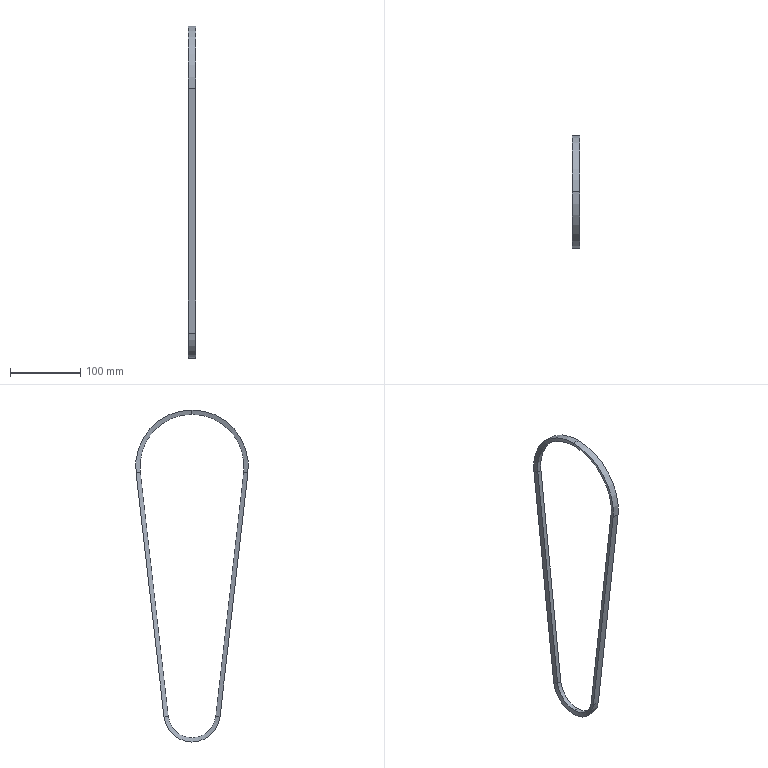Part | SolidWorks | features Sweep 1 | 1 solid | 22 faces | box 10 x 160 x 471.5 mm | volume 52282 mm3 | cylinder 8 | plane 8 | cone 6 | commonest cylinder face diameters 68 x2 80 x2 148 x2 160 x2
STEP:
#1=CARTESIAN_POINT('',(3.166,0.,74.));
#2=VERTEX_POINT('',#1);
#3=CARTESIAN_POINT('',(3.166,73.519,-8.421));
#4=VERTEX_POINT('',#3);
#5=CARTESIAN_POINT('',(3.166,0.,0.));
#6=DIRECTION('',(-1.,0.,0.));
#7=DIRECTION('',(0.,0.,1.));
#8=AXIS2_PLACEMENT_3D('',#5,#6,#7);
#9=CIRCLE('',#8,74.);
#10=EDGE_CURVE('',#2,#4,#9,.T.);
#11=ORIENTED_EDGE('',*,*,#10,.F.);
#12=CARTESIAN_POINT('',(-3.166,0.,74.));
#13=VERTEX_POINT('',#12);
#14=CARTESIAN_POINT('',(0.,0.,74.));
#15=DIRECTION('',(-1.,0.,0.));
#16=VECTOR('',#15,1000.);
#17=LINE('',#14,#16);
#18=EDGE_CURVE('',#2,#13,#17,.T.);
#19=ORIENTED_EDGE('',*,*,#18,.T.);
#20=CARTESIAN_POINT('',(-3.166,73.519,-8.421));
#21=VERTEX_POINT('',#20);
#22=CARTESIAN_POINT('',(-3.166,0.,0.));
#23=DIRECTION('',(-1.,0.,0.));
#24=DIRECTION('',(0.,0.,1.));
#25=AXIS2_PLACEMENT_3D('',#22,#23,#24);
#26=CIRCLE('',#25,74.);
#27=EDGE_CURVE('',#13,#21,#26,.T.);
#28=ORIENTED_EDGE('',*,*,#27,.T.);
#29=CARTESIAN_POINT('',(3.166,73.519,-8.421));
#30=DIRECTION('',(1.,0.,0.));
#31=VECTOR('',#30,1000.);
#32=LINE('',#29,#31);
#33=EDGE_CURVE('',#21,#4,#32,.T.);
#34=ORIENTED_EDGE('',*,*,#33,.T.);
#35=EDGE_LOOP('',(#11,#19,#28,#34));
#36=FACE_OUTER_BOUND('',#35,.T.);
#37=CARTESIAN_POINT('',(0.,0.,0.));
#38=DIRECTION('',(-1.,0.,0.));
#39=DIRECTION('',(0.,0.,1.));
#40=AXIS2_PLACEMENT_3D('',#37,#38,#39);
#41=CYLINDRICAL_SURFACE('',#40,74.);
#42=ADVANCED_FACE('',(#36),#41,.F.);
#43=CARTESIAN_POINT('',(5.,-79.48,-9.104));
#44=VERTEX_POINT('',#43);
#45=CARTESIAN_POINT('',(5.,0.,80.));
#46=VERTEX_POINT('',#45);
#47=CARTESIAN_POINT('',(5.,0.,0.));
#48=DIRECTION('',(-1.,0.,0.));
#49=DIRECTION('',(0.,0.,1.));
#50=AXIS2_PLACEMENT_3D('',#47,#48,#49);
#51=CIRCLE('',#50,80.);
#52=EDGE_CURVE('',#44,#46,#51,.T.);
#53=ORIENTED_EDGE('',*,*,#52,.T.);
#54=CARTESIAN_POINT('',(-5.,0.,80.));
#55=VERTEX_POINT('',#54);
#56=CARTESIAN_POINT('',(0.,0.,80.));
#57=DIRECTION('',(-1.,0.,0.));
#58=VECTOR('',#57,1000.);
#59=LINE('',#56,#58);
#60=EDGE_CURVE('',#46,#55,#59,.T.);
#61=ORIENTED_EDGE('',*,*,#60,.T.);
#62=CARTESIAN_POINT('',(-5.,-79.48,-9.104));
#63=VERTEX_POINT('',#62);
#64=CARTESIAN_POINT('',(-5.,0.,0.));
#65=DIRECTION('',(-1.,0.,0.));
#66=DIRECTION('',(0.,0.,1.));
#67=AXIS2_PLACEMENT_3D('',#64,#65,#66);
#68=CIRCLE('',#67,80.);
#69=EDGE_CURVE('',#63,#55,#68,.T.);
#70=ORIENTED_EDGE('',*,*,#69,.F.);
#71=CARTESIAN_POINT('',(-5.,-79.48,-9.104));
#72=DIRECTION('',(-1.,0.,0.));
#73=VECTOR('',#72,1000.);
#74=LINE('',#71,#73);
#75=EDGE_CURVE('',#44,#63,#74,.T.);
#76=ORIENTED_EDGE('',*,*,#75,.F.);
#77=EDGE_LOOP('',(#53,#61,#70,#76));
#78=FACE_OUTER_BOUND('',#77,.T.);
#79=CARTESIAN_POINT('',(0.,0.,0.));
#80=DIRECTION('',(-1.,0.,0.));
#81=DIRECTION('',(0.,0.,1.));
#82=AXIS2_PLACEMENT_3D('',#79,#80,#81);
#83=CYLINDRICAL_SURFACE('',#82,80.);
#84=ADVANCED_FACE('',(#78),#83,.T.);
#85=ORIENTED_EDGE('',*,*,#27,.F.);
#86=CARTESIAN_POINT('',(-5.,0.,80.));
#87=DIRECTION('',(-0.2924,0.,0.9563));
#88=VECTOR('',#87,1000.);
#89=LINE('',#86,#88);
#90=EDGE_CURVE('',#13,#55,#89,.T.);
#91=ORIENTED_EDGE('',*,*,#90,.T.);
#92=CARTESIAN_POINT('',(-5.,79.48,-9.104));
#93=VERTEX_POINT('',#92);
#94=CARTESIAN_POINT('',(-5.,0.,0.));
#95=DIRECTION('',(-1.,0.,0.));
#96=DIRECTION('',(0.,0.,1.));
#97=AXIS2_PLACEMENT_3D('',#94,#95,#96);
#98=CIRCLE('',#97,80.);
#99=EDGE_CURVE('',#55,#93,#98,.T.);
#100=ORIENTED_EDGE('',*,*,#99,.T.);
#101=CARTESIAN_POINT('',(-3.166,73.519,-8.421));
#102=DIRECTION('',(0.2924,-0.9501,0.1088));
#103=VECTOR('',#102,1000.);
#104=LINE('',#101,#103);
#105=EDGE_CURVE('',#93,#21,#104,.T.);
#106=ORIENTED_EDGE('',*,*,#105,.T.);
#107=EDGE_LOOP('',(#85,#91,#100,#106));
#108=FACE_OUTER_BOUND('',#107,.T.);
#109=CARTESIAN_POINT('',(-5.,0.,0.));
#110=DIRECTION('',(-1.,0.,0.));
#111=DIRECTION('',(0.,0.,1.));
#112=AXIS2_PLACEMENT_3D('',#109,#110,#111);
#113=CONICAL_SURFACE('',#112,80.,1.274);
#114=ADVANCED_FACE('',(#108),#113,.F.);
#115=CARTESIAN_POINT('',(-5.,-39.74,-356.052));
#116=VERTEX_POINT('',#115);
#117=CARTESIAN_POINT('',(-5.,0.,-391.5));
#118=VERTEX_POINT('',#117);
#119=CARTESIAN_POINT('',(-5.,0.,-351.5));
#120=DIRECTION('',(1.,0.,0.));
#121=DIRECTION('',(0.,0.,-1.));
#122=AXIS2_PLACEMENT_3D('',#119,#120,#121);
#123=CIRCLE('',#122,40.);
#124=EDGE_CURVE('',#116,#118,#123,.T.);
#125=ORIENTED_EDGE('',*,*,#124,.T.);
#126=CARTESIAN_POINT('',(5.,0.,-391.5));
#127=VERTEX_POINT('',#126);
#128=CARTESIAN_POINT('',(0.,0.,-391.5));
#129=DIRECTION('',(1.,0.,0.));
#130=VECTOR('',#129,1000.);
#131=LINE('',#128,#130);
#132=EDGE_CURVE('',#118,#127,#131,.T.);
#133=ORIENTED_EDGE('',*,*,#132,.T.);
#134=CARTESIAN_POINT('',(5.,-39.74,-356.052));
#135=VERTEX_POINT('',#134);
#136=CARTESIAN_POINT('',(5.,0.,-351.5));
#137=DIRECTION('',(1.,0.,0.));
#138=DIRECTION('',(0.,0.,-1.));
#139=AXIS2_PLACEMENT_3D('',#136,#137,#138);
#140=CIRCLE('',#139,40.);
#141=EDGE_CURVE('',#135,#127,#140,.T.);
#142=ORIENTED_EDGE('',*,*,#141,.F.);
#143=CARTESIAN_POINT('',(-5.,-39.74,-356.052));
#144=DIRECTION('',(-1.,0.,0.));
#145=VECTOR('',#144,1000.);
#146=LINE('',#143,#145);
#147=EDGE_CURVE('',#135,#116,#146,.T.);
#148=ORIENTED_EDGE('',*,*,#147,.T.);
#149=EDGE_LOOP('',(#125,#133,#142,#148));
#150=FACE_OUTER_BOUND('',#149,.T.);
#151=CARTESIAN_POINT('',(0.,0.,-351.5));
#152=DIRECTION('',(1.,0.,0.));
#153=DIRECTION('',(0.,0.,-1.));
#154=AXIS2_PLACEMENT_3D('',#151,#152,#153);
#155=CYLINDRICAL_SURFACE('',#154,40.);
#156=ADVANCED_FACE('',(#150),#155,.T.);
#157=CARTESIAN_POINT('',(3.166,0.,-385.5));
#158=VERTEX_POINT('',#157);
#159=CARTESIAN_POINT('',(3.166,33.779,-355.369));
#160=VERTEX_POINT('',#159);
#161=CARTESIAN_POINT('',(3.166,0.,-351.5));
#162=DIRECTION('',(1.,0.,0.));
#163=DIRECTION('',(0.,0.,-1.));
#164=AXIS2_PLACEMENT_3D('',#161,#162,#163);
#165=CIRCLE('',#164,34.);
#166=EDGE_CURVE('',#158,#160,#165,.T.);
#167=ORIENTED_EDGE('',*,*,#166,.F.);
#168=CARTESIAN_POINT('',(3.166,0.,-385.5));
#169=DIRECTION('',(0.2924,0.,-0.9563));
#170=VECTOR('',#169,1000.);
#171=LINE('',#168,#170);
#172=EDGE_CURVE('',#158,#127,#171,.T.);
#173=ORIENTED_EDGE('',*,*,#172,.T.);
#174=CARTESIAN_POINT('',(5.,39.74,-356.052));
#175=VERTEX_POINT('',#174);
#176=CARTESIAN_POINT('',(5.,0.,-351.5));
#177=DIRECTION('',(1.,0.,0.));
#178=DIRECTION('',(0.,0.,-1.));
#179=AXIS2_PLACEMENT_3D('',#176,#177,#178);
#180=CIRCLE('',#179,40.);
#181=EDGE_CURVE('',#127,#175,#180,.T.);
#182=ORIENTED_EDGE('',*,*,#181,.T.);
#183=CARTESIAN_POINT('',(5.,39.74,-356.052));
#184=DIRECTION('',(0.2924,0.9501,-0.1088));
#185=VECTOR('',#184,1000.);
#186=LINE('',#183,#185);
#187=EDGE_CURVE('',#160,#175,#186,.T.);
#188=ORIENTED_EDGE('',*,*,#187,.F.);
#189=EDGE_LOOP('',(#167,#173,#182,#188));
#190=FACE_OUTER_BOUND('',#189,.T.);
#191=CARTESIAN_POINT('',(3.166,0.,-351.5));
#192=DIRECTION('',(1.,0.,0.));
#193=DIRECTION('',(0.,0.,-1.));
#194=AXIS2_PLACEMENT_3D('',#191,#192,#193);
#195=CONICAL_SURFACE('',#194,34.,1.274);
#196=ADVANCED_FACE('',(#190),#195,.F.);
#197=CARTESIAN_POINT('',(-3.166,0.,-385.5));
#198=VERTEX_POINT('',#197);
#199=CARTESIAN_POINT('',(-3.166,33.779,-355.369));
#200=VERTEX_POINT('',#199);
#201=CARTESIAN_POINT('',(-3.166,0.,-351.5));
#202=DIRECTION('',(1.,0.,0.));
#203=DIRECTION('',(0.,0.,-1.));
#204=AXIS2_PLACEMENT_3D('',#201,#202,#203);
#205=CIRCLE('',#204,34.);
#206=EDGE_CURVE('',#198,#200,#205,.T.);
#207=ORIENTED_EDGE('',*,*,#206,.F.);
#208=CARTESIAN_POINT('',(0.,0.,-385.5));
#209=DIRECTION('',(1.,0.,0.));
#210=VECTOR('',#209,1000.);
#211=LINE('',#208,#210);
#212=EDGE_CURVE('',#198,#158,#211,.T.);
#213=ORIENTED_EDGE('',*,*,#212,.T.);
#214=ORIENTED_EDGE('',*,*,#166,.T.);
#215=CARTESIAN_POINT('',(3.166,33.779,-355.369));
#216=DIRECTION('',(1.,0.,0.));
#217=VECTOR('',#216,1000.);
#218=LINE('',#215,#217);
#219=EDGE_CURVE('',#200,#160,#218,.T.);
#220=ORIENTED_EDGE('',*,*,#219,.F.);
#221=EDGE_LOOP('',(#207,#213,#214,#220));
#222=FACE_OUTER_BOUND('',#221,.T.);
#223=CARTESIAN_POINT('',(0.,0.,-351.5));
#224=DIRECTION('',(1.,0.,0.));
#225=DIRECTION('',(0.,0.,-1.));
#226=AXIS2_PLACEMENT_3D('',#223,#224,#225);
#227=CYLINDRICAL_SURFACE('',#226,34.);
#228=ADVANCED_FACE('',(#222),#227,.F.);
#229=ORIENTED_EDGE('',*,*,#219,.T.);
#230=CARTESIAN_POINT('',(3.166,33.779,-355.369));
#231=DIRECTION('',(0.,0.1138,0.9935));
#232=VECTOR('',#231,1000.);
#233=LINE('',#230,#232);
#234=EDGE_CURVE('',#160,#4,#233,.T.);
#235=ORIENTED_EDGE('',*,*,#234,.T.);
#236=ORIENTED_EDGE('',*,*,#33,.F.);
#237=CARTESIAN_POINT('',(-3.166,33.779,-355.369));
#238=DIRECTION('',(0.,0.1138,0.9935));
#239=VECTOR('',#238,1000.);
#240=LINE('',#237,#239);
#241=EDGE_CURVE('',#200,#21,#240,.T.);
#242=ORIENTED_EDGE('',*,*,#241,.F.);
#243=EDGE_LOOP('',(#229,#235,#236,#242));
#244=FACE_OUTER_BOUND('',#243,.T.);
#245=CARTESIAN_POINT('',(3.166,33.779,-355.369));
#246=DIRECTION('',(0.,-0.9935,0.1138));
#247=DIRECTION('',(0.,-0.1138,-0.9935));
#248=AXIS2_PLACEMENT_3D('',#245,#246,#247);
#249=PLANE('',#248);
#250=ADVANCED_FACE('',(#244),#249,.T.);
#251=ORIENTED_EDGE('',*,*,#187,.T.);
#252=CARTESIAN_POINT('',(5.,79.48,-9.104));
#253=VERTEX_POINT('',#252);
#254=CARTESIAN_POINT('',(5.,39.74,-356.052));
#255=DIRECTION('',(0.,0.1138,0.9935));
#256=VECTOR('',#255,1000.);
#257=LINE('',#254,#256);
#258=EDGE_CURVE('',#175,#253,#257,.T.);
#259=ORIENTED_EDGE('',*,*,#258,.T.);
#260=CARTESIAN_POINT('',(5.,79.48,-9.104));
#261=DIRECTION('',(0.2924,0.9501,-0.1088));
#262=VECTOR('',#261,1000.);
#263=LINE('',#260,#262);
#264=EDGE_CURVE('',#4,#253,#263,.T.);
#265=ORIENTED_EDGE('',*,*,#264,.F.);
#266=ORIENTED_EDGE('',*,*,#234,.F.);
#267=EDGE_LOOP('',(#251,#259,#265,#266));
#268=FACE_OUTER_BOUND('',#267,.T.);
#269=CARTESIAN_POINT('',(5.,39.74,-356.052));
#270=DIRECTION('',(0.9563,-0.2905,0.03327));
#271=DIRECTION('',(0.2906,0.9568,0.));
#272=AXIS2_PLACEMENT_3D('',#269,#270,#271);
#273=PLANE('',#272);
#274=ADVANCED_FACE('',(#268),#273,.T.);
#275=CARTESIAN_POINT('',(-5.,39.74,-356.052));
#276=VERTEX_POINT('',#275);
#277=CARTESIAN_POINT('',(-5.,39.74,-356.052));
#278=DIRECTION('',(-1.,0.,0.));
#279=VECTOR('',#278,1000.);
#280=LINE('',#277,#279);
#281=EDGE_CURVE('',#175,#276,#280,.T.);
#282=ORIENTED_EDGE('',*,*,#281,.T.);
#283=CARTESIAN_POINT('',(-5.,39.74,-356.052));
#284=DIRECTION('',(0.,0.1138,0.9935));
#285=VECTOR('',#284,1000.);
#286=LINE('',#283,#285);
#287=EDGE_CURVE('',#276,#93,#286,.T.);
#288=ORIENTED_EDGE('',*,*,#287,.T.);
#289=CARTESIAN_POINT('',(-5.,79.48,-9.104));
#290=DIRECTION('',(-1.,0.,0.));
#291=VECTOR('',#290,1000.);
#292=LINE('',#289,#291);
#293=EDGE_CURVE('',#253,#93,#292,.T.);
#294=ORIENTED_EDGE('',*,*,#293,.F.);
#295=ORIENTED_EDGE('',*,*,#258,.F.);
#296=EDGE_LOOP('',(#282,#288,#294,#295));
#297=FACE_OUTER_BOUND('',#296,.T.);
#298=CARTESIAN_POINT('',(-5.,39.74,-356.052));
#299=DIRECTION('',(0.,0.9935,-0.1138));
#300=DIRECTION('',(0.,0.1138,0.9935));
#301=AXIS2_PLACEMENT_3D('',#298,#299,#300);
#302=PLANE('',#301);
#303=ADVANCED_FACE('',(#297),#302,.T.);
#304=CARTESIAN_POINT('',(-3.166,33.779,-355.369));
#305=DIRECTION('',(0.2924,-0.9501,0.1088));
#306=VECTOR('',#305,1000.);
#307=LINE('',#304,#306);
#308=EDGE_CURVE('',#276,#200,#307,.T.);
#309=ORIENTED_EDGE('',*,*,#308,.T.);
#310=ORIENTED_EDGE('',*,*,#241,.T.);
#311=ORIENTED_EDGE('',*,*,#105,.F.);
#312=ORIENTED_EDGE('',*,*,#287,.F.);
#313=EDGE_LOOP('',(#309,#310,#311,#312));
#314=FACE_OUTER_BOUND('',#313,.T.);
#315=CARTESIAN_POINT('',(-3.166,33.779,-355.369));
#316=DIRECTION('',(-0.9563,-0.2905,0.03327));
#317=DIRECTION('',(0.2906,-0.9568,0.));
#318=AXIS2_PLACEMENT_3D('',#315,#316,#317);
#319=PLANE('',#318);
#320=ADVANCED_FACE('',(#314),#319,.T.);
#321=ORIENTED_EDGE('',*,*,#212,.F.);
#322=CARTESIAN_POINT('',(-3.166,-33.779,-355.369));
#323=VERTEX_POINT('',#322);
#324=CARTESIAN_POINT('',(-3.166,0.,-351.5));
#325=DIRECTION('',(1.,0.,0.));
#326=DIRECTION('',(0.,0.,-1.));
#327=AXIS2_PLACEMENT_3D('',#324,#325,#326);
#328=CIRCLE('',#327,34.);
#329=EDGE_CURVE('',#323,#198,#328,.T.);
#330=ORIENTED_EDGE('',*,*,#329,.F.);
#331=CARTESIAN_POINT('',(3.166,-33.779,-355.369));
#332=VERTEX_POINT('',#331);
#333=CARTESIAN_POINT('',(3.166,-33.779,-355.369));
#334=DIRECTION('',(1.,0.,0.));
#335=VECTOR('',#334,1000.);
#336=LINE('',#333,#335);
#337=EDGE_CURVE('',#323,#332,#336,.T.);
#338=ORIENTED_EDGE('',*,*,#337,.T.);
#339=CARTESIAN_POINT('',(3.166,0.,-351.5));
#340=DIRECTION('',(1.,0.,0.));
#341=DIRECTION('',(0.,0.,-1.));
#342=AXIS2_PLACEMENT_3D('',#339,#340,#341);
#343=CIRCLE('',#342,34.);
#344=EDGE_CURVE('',#332,#158,#343,.T.);
#345=ORIENTED_EDGE('',*,*,#344,.T.);
#346=EDGE_LOOP('',(#321,#330,#338,#345));
#347=FACE_OUTER_BOUND('',#346,.T.);
#348=CARTESIAN_POINT('',(0.,0.,-351.5));
#349=DIRECTION('',(1.,0.,0.));
#350=DIRECTION('',(0.,0.,-1.));
#351=AXIS2_PLACEMENT_3D('',#348,#349,#350);
#352=CYLINDRICAL_SURFACE('',#351,34.);
#353=ADVANCED_FACE('',(#347),#352,.F.);
#354=ORIENTED_EDGE('',*,*,#172,.F.);
#355=ORIENTED_EDGE('',*,*,#344,.F.);
#356=CARTESIAN_POINT('',(5.,-39.74,-356.052));
#357=DIRECTION('',(0.2924,-0.9501,-0.1088));
#358=VECTOR('',#357,1000.);
#359=LINE('',#356,#358);
#360=EDGE_CURVE('',#332,#135,#359,.T.);
#361=ORIENTED_EDGE('',*,*,#360,.T.);
#362=ORIENTED_EDGE('',*,*,#141,.T.);
#363=EDGE_LOOP('',(#354,#355,#361,#362));
#364=FACE_OUTER_BOUND('',#363,.T.);
#365=CARTESIAN_POINT('',(3.166,0.,-351.5));
#366=DIRECTION('',(1.,0.,0.));
#367=DIRECTION('',(0.,0.,-1.));
#368=AXIS2_PLACEMENT_3D('',#365,#366,#367);
#369=CONICAL_SURFACE('',#368,34.,1.274);
#370=ADVANCED_FACE('',(#364),#369,.F.);
#371=ORIENTED_EDGE('',*,*,#132,.F.);
#372=CARTESIAN_POINT('',(-5.,0.,-351.5));
#373=DIRECTION('',(1.,0.,0.));
#374=DIRECTION('',(0.,0.,-1.));
#375=AXIS2_PLACEMENT_3D('',#372,#373,#374);
#376=CIRCLE('',#375,40.);
#377=EDGE_CURVE('',#118,#276,#376,.T.);
#378=ORIENTED_EDGE('',*,*,#377,.T.);
#379=ORIENTED_EDGE('',*,*,#281,.F.);
#380=ORIENTED_EDGE('',*,*,#181,.F.);
#381=EDGE_LOOP('',(#371,#378,#379,#380));
#382=FACE_OUTER_BOUND('',#381,.T.);
#383=CARTESIAN_POINT('',(0.,0.,-351.5));
#384=DIRECTION('',(1.,0.,0.));
#385=DIRECTION('',(0.,0.,-1.));
#386=AXIS2_PLACEMENT_3D('',#383,#384,#385);
#387=CYLINDRICAL_SURFACE('',#386,40.);
#388=ADVANCED_FACE('',(#382),#387,.T.);
#389=CARTESIAN_POINT('',(-3.166,-33.779,-355.369));
#390=DIRECTION('',(0.2924,0.9501,0.1088));
#391=VECTOR('',#390,1000.);
#392=LINE('',#389,#391);
#393=EDGE_CURVE('',#116,#323,#392,.T.);
#394=ORIENTED_EDGE('',*,*,#393,.T.);
#395=ORIENTED_EDGE('',*,*,#329,.T.);
#396=ORIENTED_EDGE('',*,*,#206,.T.);
#397=ORIENTED_EDGE('',*,*,#308,.F.);
#398=ORIENTED_EDGE('',*,*,#377,.F.);
#399=ORIENTED_EDGE('',*,*,#124,.F.);
#400=EDGE_LOOP('',(#394,#395,#396,#397,#398,#399));
#401=FACE_OUTER_BOUND('',#400,.T.);
#402=CARTESIAN_POINT('',(-5.,0.,-351.5));
#403=DIRECTION('',(-1.,0.,0.));
#404=DIRECTION('',(0.,0.,1.));
#405=AXIS2_PLACEMENT_3D('',#402,#403,#404);
#406=CONICAL_SURFACE('',#405,40.,1.274);
#407=ADVANCED_FACE('',(#401),#406,.F.);
#408=CARTESIAN_POINT('',(-3.166,-73.519,-8.421));
#409=VERTEX_POINT('',#408);
#410=CARTESIAN_POINT('',(3.166,-73.519,-8.421));
#411=VERTEX_POINT('',#410);
#412=CARTESIAN_POINT('',(3.166,-73.519,-8.421));
#413=DIRECTION('',(1.,0.,0.));
#414=VECTOR('',#413,1000.);
#415=LINE('',#412,#414);
#416=EDGE_CURVE('',#409,#411,#415,.T.);
#417=ORIENTED_EDGE('',*,*,#416,.T.);
#418=CARTESIAN_POINT('',(3.166,-73.519,-8.421));
#419=DIRECTION('',(0.,0.1138,-0.9935));
#420=VECTOR('',#419,1000.);
#421=LINE('',#418,#420);
#422=EDGE_CURVE('',#411,#332,#421,.T.);
#423=ORIENTED_EDGE('',*,*,#422,.T.);
#424=ORIENTED_EDGE('',*,*,#337,.F.);
#425=CARTESIAN_POINT('',(-3.166,-73.519,-8.421));
#426=DIRECTION('',(0.,0.1138,-0.9935));
#427=VECTOR('',#426,1000.);
#428=LINE('',#425,#427);
#429=EDGE_CURVE('',#409,#323,#428,.T.);
#430=ORIENTED_EDGE('',*,*,#429,.F.);
#431=EDGE_LOOP('',(#417,#423,#424,#430));
#432=FACE_OUTER_BOUND('',#431,.T.);
#433=CARTESIAN_POINT('',(3.166,-73.519,-8.421));
#434=DIRECTION('',(0.,0.9935,0.1138));
#435=DIRECTION('',(0.,-0.1138,0.9935));
#436=AXIS2_PLACEMENT_3D('',#433,#434,#435);
#437=PLANE('',#436);
#438=ADVANCED_FACE('',(#432),#437,.T.);
#439=CARTESIAN_POINT('',(5.,-79.48,-9.104));
#440=DIRECTION('',(0.2924,-0.9501,-0.1088));
#441=VECTOR('',#440,1000.);
#442=LINE('',#439,#441);
#443=EDGE_CURVE('',#411,#44,#442,.T.);
#444=ORIENTED_EDGE('',*,*,#443,.T.);
#445=CARTESIAN_POINT('',(5.,-79.48,-9.104));
#446=DIRECTION('',(0.,0.1138,-0.9935));
#447=VECTOR('',#446,1000.);
#448=LINE('',#445,#447);
#449=EDGE_CURVE('',#44,#135,#448,.T.);
#450=ORIENTED_EDGE('',*,*,#449,.T.);
#451=ORIENTED_EDGE('',*,*,#360,.F.);
#452=ORIENTED_EDGE('',*,*,#422,.F.);
#453=EDGE_LOOP('',(#444,#450,#451,#452));
#454=FACE_OUTER_BOUND('',#453,.T.);
#455=CARTESIAN_POINT('',(5.,-79.48,-9.104));
#456=DIRECTION('',(0.9563,0.2905,0.03327));
#457=DIRECTION('',(-0.2906,0.9568,0.));
#458=AXIS2_PLACEMENT_3D('',#455,#456,#457);
#459=PLANE('',#458);
#460=ADVANCED_FACE('',(#454),#459,.T.);
#461=ORIENTED_EDGE('',*,*,#75,.T.);
#462=CARTESIAN_POINT('',(-5.,-79.48,-9.104));
#463=DIRECTION('',(0.,0.1138,-0.9935));
#464=VECTOR('',#463,1000.);
#465=LINE('',#462,#464);
#466=EDGE_CURVE('',#63,#116,#465,.T.);
#467=ORIENTED_EDGE('',*,*,#466,.T.);
#468=ORIENTED_EDGE('',*,*,#147,.F.);
#469=ORIENTED_EDGE('',*,*,#449,.F.);
#470=EDGE_LOOP('',(#461,#467,#468,#469));
#471=FACE_OUTER_BOUND('',#470,.T.);
#472=CARTESIAN_POINT('',(-5.,-79.48,-9.104));
#473=DIRECTION('',(0.,-0.9935,-0.1138));
#474=DIRECTION('',(0.,0.1138,-0.9935));
#475=AXIS2_PLACEMENT_3D('',#472,#473,#474);
#476=PLANE('',#475);
#477=ADVANCED_FACE('',(#471),#476,.T.);
#478=CARTESIAN_POINT('',(-3.166,-73.519,-8.421));
#479=DIRECTION('',(0.2924,0.9501,0.1088));
#480=VECTOR('',#479,1000.);
#481=LINE('',#478,#480);
#482=EDGE_CURVE('',#63,#409,#481,.T.);
#483=ORIENTED_EDGE('',*,*,#482,.T.);
#484=ORIENTED_EDGE('',*,*,#429,.T.);
#485=ORIENTED_EDGE('',*,*,#393,.F.);
#486=ORIENTED_EDGE('',*,*,#466,.F.);
#487=EDGE_LOOP('',(#483,#484,#485,#486));
#488=FACE_OUTER_BOUND('',#487,.T.);
#489=CARTESIAN_POINT('',(-3.166,-73.519,-8.421));
#490=DIRECTION('',(-0.9563,0.2905,0.03327));
#491=DIRECTION('',(-0.2906,-0.9568,0.));
#492=AXIS2_PLACEMENT_3D('',#489,#490,#491);
#493=PLANE('',#492);
#494=ADVANCED_FACE('',(#488),#493,.T.);
#495=ORIENTED_EDGE('',*,*,#90,.F.);
#496=CARTESIAN_POINT('',(-3.166,0.,0.));
#497=DIRECTION('',(-1.,0.,0.));
#498=DIRECTION('',(0.,0.,1.));
#499=AXIS2_PLACEMENT_3D('',#496,#497,#498);
#500=CIRCLE('',#499,74.);
#501=EDGE_CURVE('',#409,#13,#500,.T.);
#502=ORIENTED_EDGE('',*,*,#501,.F.);
#503=ORIENTED_EDGE('',*,*,#482,.F.);
#504=ORIENTED_EDGE('',*,*,#69,.T.);
#505=EDGE_LOOP('',(#495,#502,#503,#504));
#506=FACE_OUTER_BOUND('',#505,.T.);
#507=CARTESIAN_POINT('',(-5.,0.,0.));
#508=DIRECTION('',(-1.,0.,0.));
#509=DIRECTION('',(0.,0.,1.));
#510=AXIS2_PLACEMENT_3D('',#507,#508,#509);
#511=CONICAL_SURFACE('',#510,80.,1.274);
#512=ADVANCED_FACE('',(#506),#511,.F.);
#513=ORIENTED_EDGE('',*,*,#60,.F.);
#514=CARTESIAN_POINT('',(5.,0.,0.));
#515=DIRECTION('',(-1.,0.,0.));
#516=DIRECTION('',(0.,0.,1.));
#517=AXIS2_PLACEMENT_3D('',#514,#515,#516);
#518=CIRCLE('',#517,80.);
#519=EDGE_CURVE('',#46,#253,#518,.T.);
#520=ORIENTED_EDGE('',*,*,#519,.T.);
#521=ORIENTED_EDGE('',*,*,#293,.T.);
#522=ORIENTED_EDGE('',*,*,#99,.F.);
#523=EDGE_LOOP('',(#513,#520,#521,#522));
#524=FACE_OUTER_BOUND('',#523,.T.);
#525=CARTESIAN_POINT('',(0.,0.,0.));
#526=DIRECTION('',(-1.,0.,0.));
#527=DIRECTION('',(0.,0.,1.));
#528=AXIS2_PLACEMENT_3D('',#525,#526,#527);
#529=CYLINDRICAL_SURFACE('',#528,80.);
#530=ADVANCED_FACE('',(#524),#529,.T.);
#531=CARTESIAN_POINT('',(3.166,0.,0.));
#532=DIRECTION('',(-1.,0.,0.));
#533=DIRECTION('',(0.,0.,1.));
#534=AXIS2_PLACEMENT_3D('',#531,#532,#533);
#535=CIRCLE('',#534,74.);
#536=EDGE_CURVE('',#411,#2,#535,.T.);
#537=ORIENTED_EDGE('',*,*,#536,.T.);
#538=ORIENTED_EDGE('',*,*,#10,.T.);
#539=ORIENTED_EDGE('',*,*,#264,.T.);
#540=ORIENTED_EDGE('',*,*,#519,.F.);
#541=ORIENTED_EDGE('',*,*,#52,.F.);
#542=ORIENTED_EDGE('',*,*,#443,.F.);
#543=EDGE_LOOP('',(#537,#538,#539,#540,#541,#542));
#544=FACE_OUTER_BOUND('',#543,.T.);
#545=CARTESIAN_POINT('',(3.166,0.,0.));
#546=DIRECTION('',(1.,0.,0.));
#547=DIRECTION('',(0.,0.,-1.));
#548=AXIS2_PLACEMENT_3D('',#545,#546,#547);
#549=CONICAL_SURFACE('',#548,74.,1.274);
#550=ADVANCED_FACE('',(#544),#549,.F.);
#551=ORIENTED_EDGE('',*,*,#18,.F.);
#552=ORIENTED_EDGE('',*,*,#536,.F.);
#553=ORIENTED_EDGE('',*,*,#416,.F.);
#554=ORIENTED_EDGE('',*,*,#501,.T.);
#555=EDGE_LOOP('',(#551,#552,#553,#554));
#556=FACE_OUTER_BOUND('',#555,.T.);
#557=CARTESIAN_POINT('',(0.,0.,0.));
#558=DIRECTION('',(-1.,0.,0.));
#559=DIRECTION('',(0.,0.,1.));
#560=AXIS2_PLACEMENT_3D('',#557,#558,#559);
#561=CYLINDRICAL_SURFACE('',#560,74.);
#562=ADVANCED_FACE('',(#556),#561,.F.);
#563=CLOSED_SHELL('',(#42,#84,#114,#156,#196,#228,#250,#274,#303,#320,#353,#370,#388,#407,#438,#460,#477,#494,#512,#530,#550,#562));
#564=MANIFOLD_SOLID_BREP('',#563);
#565=CARTESIAN_POINT('',(0.,0.,0.));
#566=DIRECTION('',(0.,0.,1.));
#567=DIRECTION('',(1.,0.,0.));
#568=AXIS2_PLACEMENT_3D('',#565,#566,#567);
#569=(LENGTH_UNIT()NAMED_UNIT(*)SI_UNIT(.MILLI.,.METRE.));
#570=UNCERTAINTY_MEASURE_WITH_UNIT(LENGTH_MEASURE(0.00001),#569,'','');
#571=(NAMED_UNIT(*)PLANE_ANGLE_UNIT()SI_UNIT($,.RADIAN.));
#572=(NAMED_UNIT(*)SI_UNIT($,.STERADIAN.)SOLID_ANGLE_UNIT());
#573=(GEOMETRIC_REPRESENTATION_CONTEXT(3)GLOBAL_UNCERTAINTY_ASSIGNED_CONTEXT((#570))GLOBAL_UNIT_ASSIGNED_CONTEXT((#569,#571,#572))REPRESENTATION_CONTEXT('',''));
#574=ADVANCED_BREP_SHAPE_REPRESENTATION('',(#564,#568),#573);